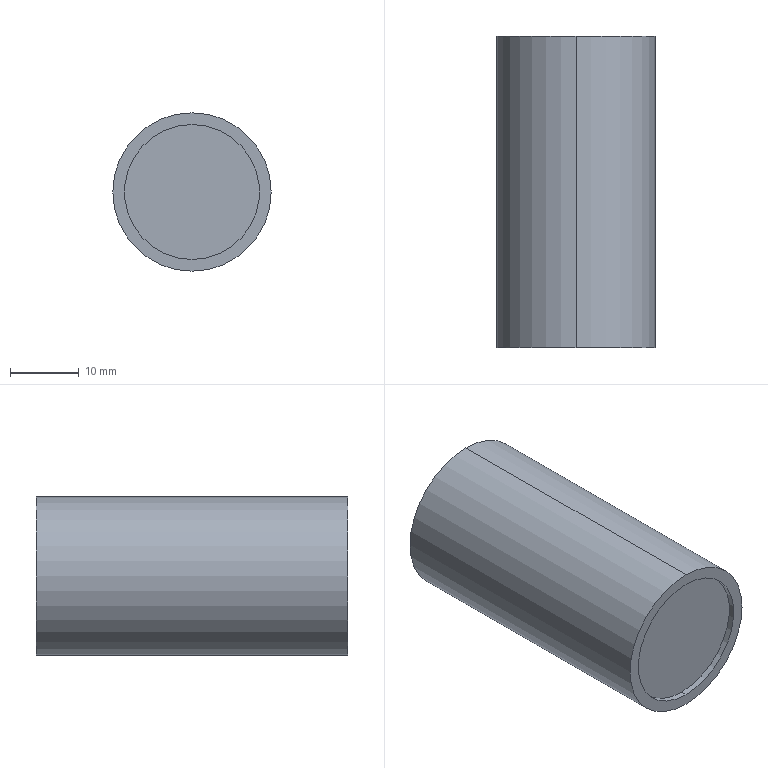Part | SolidWorks | features ICE 4, Dome 1, Extrusion 1, Shell 1 | 1 solid | 10 faces | box 23 x 45.2 x 23 mm | volume 3843 mm3 | cylinder 6 | plane 4 | commonest cylinder face diameters 19.6 x2 20.6 x2 23 x2
STEP:
#1=CARTESIAN_POINT('',(0.,0.9,9.8));
#2=VERTEX_POINT('',#1);
#3=CARTESIAN_POINT('',(0.,0.9,-9.8));
#4=VERTEX_POINT('',#3);
#5=CARTESIAN_POINT('',(0.,0.9,0.));
#6=DIRECTION('',(0.,-1.,0.));
#7=DIRECTION('',(0.,0.,-1.));
#8=AXIS2_PLACEMENT_3D('',#5,#6,#7);
#9=CIRCLE('',#8,9.8);
#10=EDGE_CURVE('',#2,#4,#9,.T.);
#11=ORIENTED_EDGE('',*,*,#10,.F.);
#12=CARTESIAN_POINT('',(0.,0.,9.8));
#13=VERTEX_POINT('',#12);
#14=CARTESIAN_POINT('',(0.,0.9,9.8));
#15=DIRECTION('',(0.,-1.,0.));
#16=VECTOR('',#15,1000.);
#17=LINE('',#14,#16);
#18=EDGE_CURVE('',#2,#13,#17,.T.);
#19=ORIENTED_EDGE('',*,*,#18,.T.);
#20=CARTESIAN_POINT('',(0.,0.,-9.8));
#21=VERTEX_POINT('',#20);
#22=CARTESIAN_POINT('',(0.,0.,0.));
#23=DIRECTION('',(0.,-1.,0.));
#24=DIRECTION('',(0.,0.,-1.));
#25=AXIS2_PLACEMENT_3D('',#22,#23,#24);
#26=CIRCLE('',#25,9.8);
#27=EDGE_CURVE('',#13,#21,#26,.T.);
#28=ORIENTED_EDGE('',*,*,#27,.T.);
#29=CARTESIAN_POINT('',(0.,0.9,-9.8));
#30=DIRECTION('',(0.,-1.,0.));
#31=VECTOR('',#30,1000.);
#32=LINE('',#29,#31);
#33=EDGE_CURVE('',#4,#21,#32,.T.);
#34=ORIENTED_EDGE('',*,*,#33,.F.);
#35=EDGE_LOOP('',(#11,#19,#28,#34));
#36=FACE_OUTER_BOUND('',#35,.T.);
#37=CARTESIAN_POINT('',(0.,0.9,0.));
#38=DIRECTION('',(0.,-1.,0.));
#39=DIRECTION('',(0.,0.,-1.));
#40=AXIS2_PLACEMENT_3D('',#37,#38,#39);
#41=CYLINDRICAL_SURFACE('',#40,9.8);
#42=ADVANCED_FACE('',(#36),#41,.F.);
#43=CARTESIAN_POINT('',(0.,1.2,-10.3));
#44=VERTEX_POINT('',#43);
#45=CARTESIAN_POINT('',(0.,1.2,10.3));
#46=VERTEX_POINT('',#45);
#47=CARTESIAN_POINT('',(0.,1.2,0.));
#48=DIRECTION('',(0.,1.,0.));
#49=DIRECTION('',(0.,0.,1.));
#50=AXIS2_PLACEMENT_3D('',#47,#48,#49);
#51=CIRCLE('',#50,10.3);
#52=EDGE_CURVE('',#44,#46,#51,.T.);
#53=ORIENTED_EDGE('',*,*,#52,.F.);
#54=CARTESIAN_POINT('',(0.,45.2,-10.3));
#55=VERTEX_POINT('',#54);
#56=CARTESIAN_POINT('',(0.,1.2,-10.3));
#57=DIRECTION('',(0.,1.,0.));
#58=VECTOR('',#57,1000.);
#59=LINE('',#56,#58);
#60=EDGE_CURVE('',#44,#55,#59,.T.);
#61=ORIENTED_EDGE('',*,*,#60,.T.);
#62=CARTESIAN_POINT('',(0.,45.2,10.3));
#63=VERTEX_POINT('',#62);
#64=CARTESIAN_POINT('',(0.,45.2,0.));
#65=DIRECTION('',(0.,1.,0.));
#66=DIRECTION('',(0.,0.,1.));
#67=AXIS2_PLACEMENT_3D('',#64,#65,#66);
#68=CIRCLE('',#67,10.3);
#69=EDGE_CURVE('',#55,#63,#68,.T.);
#70=ORIENTED_EDGE('',*,*,#69,.T.);
#71=CARTESIAN_POINT('',(0.,1.2,10.3));
#72=DIRECTION('',(0.,1.,0.));
#73=VECTOR('',#72,1000.);
#74=LINE('',#71,#73);
#75=EDGE_CURVE('',#46,#63,#74,.T.);
#76=ORIENTED_EDGE('',*,*,#75,.F.);
#77=EDGE_LOOP('',(#53,#61,#70,#76));
#78=FACE_OUTER_BOUND('',#77,.T.);
#79=CARTESIAN_POINT('',(0.,1.2,0.));
#80=DIRECTION('',(0.,1.,0.));
#81=DIRECTION('',(0.,0.,1.));
#82=AXIS2_PLACEMENT_3D('',#79,#80,#81);
#83=CYLINDRICAL_SURFACE('',#82,10.3);
#84=ADVANCED_FACE('',(#78),#83,.F.);
#85=CARTESIAN_POINT('',(0.,45.2,11.5));
#86=VERTEX_POINT('',#85);
#87=CARTESIAN_POINT('',(0.,45.2,-11.5));
#88=VERTEX_POINT('',#87);
#89=CARTESIAN_POINT('',(0.,45.2,0.));
#90=DIRECTION('',(0.,1.,0.));
#91=DIRECTION('',(0.,0.,1.));
#92=AXIS2_PLACEMENT_3D('',#89,#90,#91);
#93=CIRCLE('',#92,11.5);
#94=EDGE_CURVE('',#86,#88,#93,.T.);
#95=ORIENTED_EDGE('',*,*,#94,.F.);
#96=CARTESIAN_POINT('',(0.,0.,11.5));
#97=VERTEX_POINT('',#96);
#98=CARTESIAN_POINT('',(0.,45.2,11.5));
#99=DIRECTION('',(0.,-1.,0.));
#100=VECTOR('',#99,1000.);
#101=LINE('',#98,#100);
#102=EDGE_CURVE('',#86,#97,#101,.T.);
#103=ORIENTED_EDGE('',*,*,#102,.T.);
#104=CARTESIAN_POINT('',(0.,0.,-11.5));
#105=VERTEX_POINT('',#104);
#106=CARTESIAN_POINT('',(0.,0.,0.));
#107=DIRECTION('',(0.,1.,0.));
#108=DIRECTION('',(0.,0.,1.));
#109=AXIS2_PLACEMENT_3D('',#106,#107,#108);
#110=CIRCLE('',#109,11.5);
#111=EDGE_CURVE('',#97,#105,#110,.T.);
#112=ORIENTED_EDGE('',*,*,#111,.T.);
#113=CARTESIAN_POINT('',(0.,45.2,-11.5));
#114=DIRECTION('',(0.,-1.,0.));
#115=VECTOR('',#114,1000.);
#116=LINE('',#113,#115);
#117=EDGE_CURVE('',#88,#105,#116,.T.);
#118=ORIENTED_EDGE('',*,*,#117,.F.);
#119=EDGE_LOOP('',(#95,#103,#112,#118));
#120=FACE_OUTER_BOUND('',#119,.T.);
#121=CARTESIAN_POINT('',(0.,45.2,0.));
#122=DIRECTION('',(0.,-1.,0.));
#123=DIRECTION('',(0.,0.,-1.));
#124=AXIS2_PLACEMENT_3D('',#121,#122,#123);
#125=CYLINDRICAL_SURFACE('',#124,11.5);
#126=ADVANCED_FACE('',(#120),#125,.T.);
#127=ORIENTED_EDGE('',*,*,#102,.F.);
#128=CARTESIAN_POINT('',(0.,45.2,0.));
#129=DIRECTION('',(0.,1.,0.));
#130=DIRECTION('',(0.,0.,1.));
#131=AXIS2_PLACEMENT_3D('',#128,#129,#130);
#132=CIRCLE('',#131,11.5);
#133=EDGE_CURVE('',#88,#86,#132,.T.);
#134=ORIENTED_EDGE('',*,*,#133,.F.);
#135=ORIENTED_EDGE('',*,*,#117,.T.);
#136=CARTESIAN_POINT('',(0.,0.,0.));
#137=DIRECTION('',(0.,1.,0.));
#138=DIRECTION('',(0.,0.,1.));
#139=AXIS2_PLACEMENT_3D('',#136,#137,#138);
#140=CIRCLE('',#139,11.5);
#141=EDGE_CURVE('',#105,#97,#140,.T.);
#142=ORIENTED_EDGE('',*,*,#141,.T.);
#143=EDGE_LOOP('',(#127,#134,#135,#142));
#144=FACE_OUTER_BOUND('',#143,.T.);
#145=CARTESIAN_POINT('',(0.,45.2,0.));
#146=DIRECTION('',(0.,-1.,0.));
#147=DIRECTION('',(0.,0.,-1.));
#148=AXIS2_PLACEMENT_3D('',#145,#146,#147);
#149=CYLINDRICAL_SURFACE('',#148,11.5);
#150=ADVANCED_FACE('',(#144),#149,.T.);
#151=CARTESIAN_POINT('',(0.,45.2,0.));
#152=DIRECTION('',(0.,1.,0.));
#153=DIRECTION('',(0.,0.,1.));
#154=AXIS2_PLACEMENT_3D('',#151,#152,#153);
#155=CIRCLE('',#154,10.3);
#156=EDGE_CURVE('',#63,#55,#155,.T.);
#157=ORIENTED_EDGE('',*,*,#156,.F.);
#158=ORIENTED_EDGE('',*,*,#69,.F.);
#159=EDGE_LOOP('',(#157,#158));
#160=FACE_BOUND('',#159,.T.);
#161=ORIENTED_EDGE('',*,*,#133,.T.);
#162=ORIENTED_EDGE('',*,*,#94,.T.);
#163=EDGE_LOOP('',(#161,#162));
#164=FACE_OUTER_BOUND('',#163,.T.);
#165=CARTESIAN_POINT('',(0.,45.2,0.));
#166=DIRECTION('',(0.,1.,0.));
#167=DIRECTION('',(0.,0.,1.));
#168=AXIS2_PLACEMENT_3D('',#165,#166,#167);
#169=PLANE('',#168);
#170=ADVANCED_FACE('',(#160,#164),#169,.T.);
#171=CARTESIAN_POINT('',(0.,0.,0.));
#172=DIRECTION('',(0.,-1.,0.));
#173=DIRECTION('',(0.,0.,-1.));
#174=AXIS2_PLACEMENT_3D('',#171,#172,#173);
#175=CIRCLE('',#174,9.8);
#176=EDGE_CURVE('',#21,#13,#175,.T.);
#177=ORIENTED_EDGE('',*,*,#176,.F.);
#178=ORIENTED_EDGE('',*,*,#27,.F.);
#179=EDGE_LOOP('',(#177,#178));
#180=FACE_BOUND('',#179,.T.);
#181=ORIENTED_EDGE('',*,*,#141,.F.);
#182=ORIENTED_EDGE('',*,*,#111,.F.);
#183=EDGE_LOOP('',(#181,#182));
#184=FACE_OUTER_BOUND('',#183,.T.);
#185=CARTESIAN_POINT('',(0.,0.,0.));
#186=DIRECTION('',(0.,1.,0.));
#187=DIRECTION('',(0.,0.,1.));
#188=AXIS2_PLACEMENT_3D('',#185,#186,#187);
#189=PLANE('',#188);
#190=ADVANCED_FACE('',(#180,#184),#189,.F.);
#191=ORIENTED_EDGE('',*,*,#60,.F.);
#192=CARTESIAN_POINT('',(0.,1.2,0.));
#193=DIRECTION('',(0.,1.,0.));
#194=DIRECTION('',(0.,0.,1.));
#195=AXIS2_PLACEMENT_3D('',#192,#193,#194);
#196=CIRCLE('',#195,10.3);
#197=EDGE_CURVE('',#46,#44,#196,.T.);
#198=ORIENTED_EDGE('',*,*,#197,.F.);
#199=ORIENTED_EDGE('',*,*,#75,.T.);
#200=ORIENTED_EDGE('',*,*,#156,.T.);
#201=EDGE_LOOP('',(#191,#198,#199,#200));
#202=FACE_OUTER_BOUND('',#201,.T.);
#203=CARTESIAN_POINT('',(0.,1.2,0.));
#204=DIRECTION('',(0.,1.,0.));
#205=DIRECTION('',(0.,0.,1.));
#206=AXIS2_PLACEMENT_3D('',#203,#204,#205);
#207=CYLINDRICAL_SURFACE('',#206,10.3);
#208=ADVANCED_FACE('',(#202),#207,.F.);
#209=ORIENTED_EDGE('',*,*,#197,.T.);
#210=ORIENTED_EDGE('',*,*,#52,.T.);
#211=EDGE_LOOP('',(#209,#210));
#212=FACE_OUTER_BOUND('',#211,.T.);
#213=CARTESIAN_POINT('',(0.,1.2,0.));
#214=DIRECTION('',(0.,1.,0.));
#215=DIRECTION('',(0.,0.,1.));
#216=AXIS2_PLACEMENT_3D('',#213,#214,#215);
#217=PLANE('',#216);
#218=ADVANCED_FACE('',(#212),#217,.T.);
#219=ORIENTED_EDGE('',*,*,#18,.F.);
#220=CARTESIAN_POINT('',(0.,0.9,0.));
#221=DIRECTION('',(0.,-1.,0.));
#222=DIRECTION('',(0.,0.,-1.));
#223=AXIS2_PLACEMENT_3D('',#220,#221,#222);
#224=CIRCLE('',#223,9.8);
#225=EDGE_CURVE('',#4,#2,#224,.T.);
#226=ORIENTED_EDGE('',*,*,#225,.F.);
#227=ORIENTED_EDGE('',*,*,#33,.T.);
#228=ORIENTED_EDGE('',*,*,#176,.T.);
#229=EDGE_LOOP('',(#219,#226,#227,#228));
#230=FACE_OUTER_BOUND('',#229,.T.);
#231=CARTESIAN_POINT('',(0.,0.9,0.));
#232=DIRECTION('',(0.,-1.,0.));
#233=DIRECTION('',(0.,0.,-1.));
#234=AXIS2_PLACEMENT_3D('',#231,#232,#233);
#235=CYLINDRICAL_SURFACE('',#234,9.8);
#236=ADVANCED_FACE('',(#230),#235,.F.);
#237=ORIENTED_EDGE('',*,*,#225,.T.);
#238=ORIENTED_EDGE('',*,*,#10,.T.);
#239=EDGE_LOOP('',(#237,#238));
#240=FACE_OUTER_BOUND('',#239,.T.);
#241=CARTESIAN_POINT('',(0.,0.9,0.));
#242=DIRECTION('',(0.,-1.,0.));
#243=DIRECTION('',(0.,0.,-1.));
#244=AXIS2_PLACEMENT_3D('',#241,#242,#243);
#245=PLANE('',#244);
#246=ADVANCED_FACE('',(#240),#245,.T.);
#247=CLOSED_SHELL('',(#42,#84,#126,#150,#170,#190,#208,#218,#236,#246));
#248=MANIFOLD_SOLID_BREP('',#247);
#249=CARTESIAN_POINT('',(0.,0.,0.));
#250=DIRECTION('',(0.,0.,1.));
#251=DIRECTION('',(1.,0.,0.));
#252=AXIS2_PLACEMENT_3D('',#249,#250,#251);
#253=(LENGTH_UNIT()NAMED_UNIT(*)SI_UNIT(.MILLI.,.METRE.));
#254=UNCERTAINTY_MEASURE_WITH_UNIT(LENGTH_MEASURE(0.00001),#253,'','');
#255=(NAMED_UNIT(*)PLANE_ANGLE_UNIT()SI_UNIT($,.RADIAN.));
#256=(NAMED_UNIT(*)SI_UNIT($,.STERADIAN.)SOLID_ANGLE_UNIT());
#257=(GEOMETRIC_REPRESENTATION_CONTEXT(3)GLOBAL_UNCERTAINTY_ASSIGNED_CONTEXT((#254))GLOBAL_UNIT_ASSIGNED_CONTEXT((#253,#255,#256))REPRESENTATION_CONTEXT('',''));
#258=ADVANCED_BREP_SHAPE_REPRESENTATION('',(#248,#252),#257);